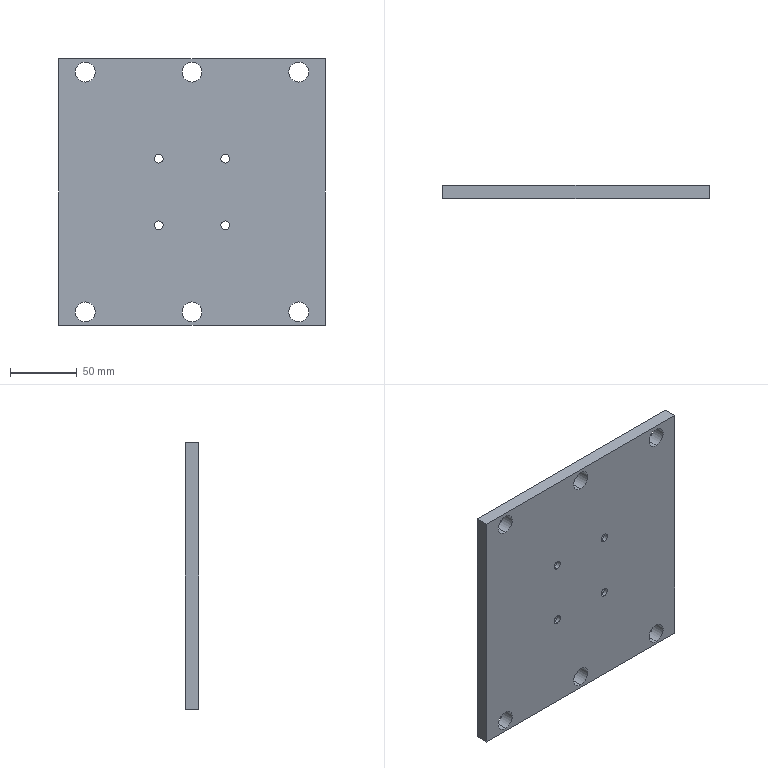Part | SolidWorks | features Extrusion 1, HoleWzd 1, ICE 1, LPattern 1 | 1 solid | 38 faces | box 200 x 10 x 200 mm | volume 386374 mm3 | cylinder 28 | plane 10 | commonest cylinder face diameters 15 x12 6.6 x8 11 x8
STEP:
#1=CARTESIAN_POINT('',(25.,-1.8,-30.5));
#2=VERTEX_POINT('',#1);
#3=CARTESIAN_POINT('',(25.,-1.8,-19.5));
#4=VERTEX_POINT('',#3);
#5=CARTESIAN_POINT('',(25.,-1.8,-25.));
#6=DIRECTION('',(0.,1.,0.));
#7=DIRECTION('',(0.,0.,1.));
#8=AXIS2_PLACEMENT_3D('',#5,#6,#7);
#9=CIRCLE('',#8,5.5);
#10=EDGE_CURVE('',#2,#4,#9,.T.);
#11=ORIENTED_EDGE('',*,*,#10,.F.);
#12=CARTESIAN_POINT('',(25.,5.,-30.5));
#13=VERTEX_POINT('',#12);
#14=CARTESIAN_POINT('',(25.,5.,-30.5));
#15=DIRECTION('',(0.,1.,0.));
#16=VECTOR('',#15,1000.);
#17=LINE('',#14,#16);
#18=EDGE_CURVE('',#2,#13,#17,.T.);
#19=ORIENTED_EDGE('',*,*,#18,.T.);
#20=CARTESIAN_POINT('',(25.,5.,-19.5));
#21=VERTEX_POINT('',#20);
#22=CARTESIAN_POINT('',(25.,5.,-25.));
#23=DIRECTION('',(0.,1.,0.));
#24=DIRECTION('',(0.,0.,1.));
#25=AXIS2_PLACEMENT_3D('',#22,#23,#24);
#26=CIRCLE('',#25,5.5);
#27=EDGE_CURVE('',#13,#21,#26,.T.);
#28=ORIENTED_EDGE('',*,*,#27,.T.);
#29=CARTESIAN_POINT('',(25.,5.,-19.5));
#30=DIRECTION('',(0.,1.,0.));
#31=VECTOR('',#30,1000.);
#32=LINE('',#29,#31);
#33=EDGE_CURVE('',#4,#21,#32,.T.);
#34=ORIENTED_EDGE('',*,*,#33,.F.);
#35=EDGE_LOOP('',(#11,#19,#28,#34));
#36=FACE_OUTER_BOUND('',#35,.T.);
#37=CARTESIAN_POINT('',(25.,5.,-25.));
#38=DIRECTION('',(0.,1.,0.));
#39=DIRECTION('',(0.,0.,1.));
#40=AXIS2_PLACEMENT_3D('',#37,#38,#39);
#41=CYLINDRICAL_SURFACE('',#40,5.5);
#42=ADVANCED_FACE('',(#36),#41,.F.);
#43=CARTESIAN_POINT('',(25.,-5.,-28.3));
#44=VERTEX_POINT('',#43);
#45=CARTESIAN_POINT('',(25.,-5.,-21.7));
#46=VERTEX_POINT('',#45);
#47=CARTESIAN_POINT('',(25.,-5.,-25.));
#48=DIRECTION('',(0.,1.,0.));
#49=DIRECTION('',(0.,0.,1.));
#50=AXIS2_PLACEMENT_3D('',#47,#48,#49);
#51=CIRCLE('',#50,3.3);
#52=EDGE_CURVE('',#44,#46,#51,.T.);
#53=ORIENTED_EDGE('',*,*,#52,.F.);
#54=CARTESIAN_POINT('',(25.,-1.8,-28.3));
#55=VERTEX_POINT('',#54);
#56=CARTESIAN_POINT('',(25.,5.,-28.3));
#57=DIRECTION('',(0.,1.,0.));
#58=VECTOR('',#57,1000.);
#59=LINE('',#56,#58);
#60=EDGE_CURVE('',#44,#55,#59,.T.);
#61=ORIENTED_EDGE('',*,*,#60,.T.);
#62=CARTESIAN_POINT('',(25.,-1.8,-21.7));
#63=VERTEX_POINT('',#62);
#64=CARTESIAN_POINT('',(25.,-1.8,-25.));
#65=DIRECTION('',(0.,1.,0.));
#66=DIRECTION('',(0.,0.,1.));
#67=AXIS2_PLACEMENT_3D('',#64,#65,#66);
#68=CIRCLE('',#67,3.3);
#69=EDGE_CURVE('',#55,#63,#68,.T.);
#70=ORIENTED_EDGE('',*,*,#69,.T.);
#71=CARTESIAN_POINT('',(25.,5.,-21.7));
#72=DIRECTION('',(0.,1.,0.));
#73=VECTOR('',#72,1000.);
#74=LINE('',#71,#73);
#75=EDGE_CURVE('',#46,#63,#74,.T.);
#76=ORIENTED_EDGE('',*,*,#75,.F.);
#77=EDGE_LOOP('',(#53,#61,#70,#76));
#78=FACE_OUTER_BOUND('',#77,.T.);
#79=CARTESIAN_POINT('',(25.,5.,-25.));
#80=DIRECTION('',(0.,1.,0.));
#81=DIRECTION('',(0.,0.,1.));
#82=AXIS2_PLACEMENT_3D('',#79,#80,#81);
#83=CYLINDRICAL_SURFACE('',#82,3.3);
#84=ADVANCED_FACE('',(#78),#83,.F.);
#85=CARTESIAN_POINT('',(25.,-1.8,19.5));
#86=VERTEX_POINT('',#85);
#87=CARTESIAN_POINT('',(25.,-1.8,30.5));
#88=VERTEX_POINT('',#87);
#89=CARTESIAN_POINT('',(25.,-1.8,25.));
#90=DIRECTION('',(0.,1.,0.));
#91=DIRECTION('',(0.,0.,1.));
#92=AXIS2_PLACEMENT_3D('',#89,#90,#91);
#93=CIRCLE('',#92,5.5);
#94=EDGE_CURVE('',#86,#88,#93,.T.);
#95=ORIENTED_EDGE('',*,*,#94,.F.);
#96=CARTESIAN_POINT('',(25.,5.,19.5));
#97=VERTEX_POINT('',#96);
#98=CARTESIAN_POINT('',(25.,5.,19.5));
#99=DIRECTION('',(0.,1.,0.));
#100=VECTOR('',#99,1000.);
#101=LINE('',#98,#100);
#102=EDGE_CURVE('',#86,#97,#101,.T.);
#103=ORIENTED_EDGE('',*,*,#102,.T.);
#104=CARTESIAN_POINT('',(25.,5.,30.5));
#105=VERTEX_POINT('',#104);
#106=CARTESIAN_POINT('',(25.,5.,25.));
#107=DIRECTION('',(0.,1.,0.));
#108=DIRECTION('',(0.,0.,1.));
#109=AXIS2_PLACEMENT_3D('',#106,#107,#108);
#110=CIRCLE('',#109,5.5);
#111=EDGE_CURVE('',#97,#105,#110,.T.);
#112=ORIENTED_EDGE('',*,*,#111,.T.);
#113=CARTESIAN_POINT('',(25.,5.,30.5));
#114=DIRECTION('',(0.,1.,0.));
#115=VECTOR('',#114,1000.);
#116=LINE('',#113,#115);
#117=EDGE_CURVE('',#88,#105,#116,.T.);
#118=ORIENTED_EDGE('',*,*,#117,.F.);
#119=EDGE_LOOP('',(#95,#103,#112,#118));
#120=FACE_OUTER_BOUND('',#119,.T.);
#121=CARTESIAN_POINT('',(25.,5.,25.));
#122=DIRECTION('',(0.,1.,0.));
#123=DIRECTION('',(0.,0.,1.));
#124=AXIS2_PLACEMENT_3D('',#121,#122,#123);
#125=CYLINDRICAL_SURFACE('',#124,5.5);
#126=ADVANCED_FACE('',(#120),#125,.F.);
#127=CARTESIAN_POINT('',(25.,-5.,21.7));
#128=VERTEX_POINT('',#127);
#129=CARTESIAN_POINT('',(25.,-5.,28.3));
#130=VERTEX_POINT('',#129);
#131=CARTESIAN_POINT('',(25.,-5.,25.));
#132=DIRECTION('',(0.,1.,0.));
#133=DIRECTION('',(0.,0.,1.));
#134=AXIS2_PLACEMENT_3D('',#131,#132,#133);
#135=CIRCLE('',#134,3.3);
#136=EDGE_CURVE('',#128,#130,#135,.T.);
#137=ORIENTED_EDGE('',*,*,#136,.F.);
#138=CARTESIAN_POINT('',(25.,-1.8,21.7));
#139=VERTEX_POINT('',#138);
#140=CARTESIAN_POINT('',(25.,5.,21.7));
#141=DIRECTION('',(0.,1.,0.));
#142=VECTOR('',#141,1000.);
#143=LINE('',#140,#142);
#144=EDGE_CURVE('',#128,#139,#143,.T.);
#145=ORIENTED_EDGE('',*,*,#144,.T.);
#146=CARTESIAN_POINT('',(25.,-1.8,28.3));
#147=VERTEX_POINT('',#146);
#148=CARTESIAN_POINT('',(25.,-1.8,25.));
#149=DIRECTION('',(0.,1.,0.));
#150=DIRECTION('',(0.,0.,1.));
#151=AXIS2_PLACEMENT_3D('',#148,#149,#150);
#152=CIRCLE('',#151,3.3);
#153=EDGE_CURVE('',#139,#147,#152,.T.);
#154=ORIENTED_EDGE('',*,*,#153,.T.);
#155=CARTESIAN_POINT('',(25.,5.,28.3));
#156=DIRECTION('',(0.,1.,0.));
#157=VECTOR('',#156,1000.);
#158=LINE('',#155,#157);
#159=EDGE_CURVE('',#130,#147,#158,.T.);
#160=ORIENTED_EDGE('',*,*,#159,.F.);
#161=EDGE_LOOP('',(#137,#145,#154,#160));
#162=FACE_OUTER_BOUND('',#161,.T.);
#163=CARTESIAN_POINT('',(25.,5.,25.));
#164=DIRECTION('',(0.,1.,0.));
#165=DIRECTION('',(0.,0.,1.));
#166=AXIS2_PLACEMENT_3D('',#163,#164,#165);
#167=CYLINDRICAL_SURFACE('',#166,3.3);
#168=ADVANCED_FACE('',(#162),#167,.F.);
#169=CARTESIAN_POINT('',(-25.,-1.8,-30.5));
#170=VERTEX_POINT('',#169);
#171=CARTESIAN_POINT('',(-25.,-1.8,-19.5));
#172=VERTEX_POINT('',#171);
#173=CARTESIAN_POINT('',(-25.,-1.8,-25.));
#174=DIRECTION('',(0.,1.,0.));
#175=DIRECTION('',(0.,0.,1.));
#176=AXIS2_PLACEMENT_3D('',#173,#174,#175);
#177=CIRCLE('',#176,5.5);
#178=EDGE_CURVE('',#170,#172,#177,.T.);
#179=ORIENTED_EDGE('',*,*,#178,.F.);
#180=CARTESIAN_POINT('',(-25.,5.,-30.5));
#181=VERTEX_POINT('',#180);
#182=CARTESIAN_POINT('',(-25.,5.,-30.5));
#183=DIRECTION('',(0.,1.,0.));
#184=VECTOR('',#183,1000.);
#185=LINE('',#182,#184);
#186=EDGE_CURVE('',#170,#181,#185,.T.);
#187=ORIENTED_EDGE('',*,*,#186,.T.);
#188=CARTESIAN_POINT('',(-25.,5.,-19.5));
#189=VERTEX_POINT('',#188);
#190=CARTESIAN_POINT('',(-25.,5.,-25.));
#191=DIRECTION('',(0.,1.,0.));
#192=DIRECTION('',(0.,0.,1.));
#193=AXIS2_PLACEMENT_3D('',#190,#191,#192);
#194=CIRCLE('',#193,5.5);
#195=EDGE_CURVE('',#181,#189,#194,.T.);
#196=ORIENTED_EDGE('',*,*,#195,.T.);
#197=CARTESIAN_POINT('',(-25.,5.,-19.5));
#198=DIRECTION('',(0.,1.,0.));
#199=VECTOR('',#198,1000.);
#200=LINE('',#197,#199);
#201=EDGE_CURVE('',#172,#189,#200,.T.);
#202=ORIENTED_EDGE('',*,*,#201,.F.);
#203=EDGE_LOOP('',(#179,#187,#196,#202));
#204=FACE_OUTER_BOUND('',#203,.T.);
#205=CARTESIAN_POINT('',(-25.,5.,-25.));
#206=DIRECTION('',(0.,1.,0.));
#207=DIRECTION('',(0.,0.,1.));
#208=AXIS2_PLACEMENT_3D('',#205,#206,#207);
#209=CYLINDRICAL_SURFACE('',#208,5.5);
#210=ADVANCED_FACE('',(#204),#209,.F.);
#211=CARTESIAN_POINT('',(-25.,-5.,-28.3));
#212=VERTEX_POINT('',#211);
#213=CARTESIAN_POINT('',(-25.,-5.,-21.7));
#214=VERTEX_POINT('',#213);
#215=CARTESIAN_POINT('',(-25.,-5.,-25.));
#216=DIRECTION('',(0.,1.,0.));
#217=DIRECTION('',(0.,0.,1.));
#218=AXIS2_PLACEMENT_3D('',#215,#216,#217);
#219=CIRCLE('',#218,3.3);
#220=EDGE_CURVE('',#212,#214,#219,.T.);
#221=ORIENTED_EDGE('',*,*,#220,.F.);
#222=CARTESIAN_POINT('',(-25.,-1.8,-28.3));
#223=VERTEX_POINT('',#222);
#224=CARTESIAN_POINT('',(-25.,5.,-28.3));
#225=DIRECTION('',(0.,1.,0.));
#226=VECTOR('',#225,1000.);
#227=LINE('',#224,#226);
#228=EDGE_CURVE('',#212,#223,#227,.T.);
#229=ORIENTED_EDGE('',*,*,#228,.T.);
#230=CARTESIAN_POINT('',(-25.,-1.8,-21.7));
#231=VERTEX_POINT('',#230);
#232=CARTESIAN_POINT('',(-25.,-1.8,-25.));
#233=DIRECTION('',(0.,1.,0.));
#234=DIRECTION('',(0.,0.,1.));
#235=AXIS2_PLACEMENT_3D('',#232,#233,#234);
#236=CIRCLE('',#235,3.3);
#237=EDGE_CURVE('',#223,#231,#236,.T.);
#238=ORIENTED_EDGE('',*,*,#237,.T.);
#239=CARTESIAN_POINT('',(-25.,5.,-21.7));
#240=DIRECTION('',(0.,1.,0.));
#241=VECTOR('',#240,1000.);
#242=LINE('',#239,#241);
#243=EDGE_CURVE('',#214,#231,#242,.T.);
#244=ORIENTED_EDGE('',*,*,#243,.F.);
#245=EDGE_LOOP('',(#221,#229,#238,#244));
#246=FACE_OUTER_BOUND('',#245,.T.);
#247=CARTESIAN_POINT('',(-25.,5.,-25.));
#248=DIRECTION('',(0.,1.,0.));
#249=DIRECTION('',(0.,0.,1.));
#250=AXIS2_PLACEMENT_3D('',#247,#248,#249);
#251=CYLINDRICAL_SURFACE('',#250,3.3);
#252=ADVANCED_FACE('',(#246),#251,.F.);
#253=CARTESIAN_POINT('',(-25.,-1.8,19.5));
#254=VERTEX_POINT('',#253);
#255=CARTESIAN_POINT('',(-25.,-1.8,30.5));
#256=VERTEX_POINT('',#255);
#257=CARTESIAN_POINT('',(-25.,-1.8,25.));
#258=DIRECTION('',(0.,1.,0.));
#259=DIRECTION('',(0.,0.,1.));
#260=AXIS2_PLACEMENT_3D('',#257,#258,#259);
#261=CIRCLE('',#260,5.5);
#262=EDGE_CURVE('',#254,#256,#261,.T.);
#263=ORIENTED_EDGE('',*,*,#262,.F.);
#264=CARTESIAN_POINT('',(-25.,5.,19.5));
#265=VERTEX_POINT('',#264);
#266=CARTESIAN_POINT('',(-25.,5.,19.5));
#267=DIRECTION('',(0.,1.,0.));
#268=VECTOR('',#267,1000.);
#269=LINE('',#266,#268);
#270=EDGE_CURVE('',#254,#265,#269,.T.);
#271=ORIENTED_EDGE('',*,*,#270,.T.);
#272=CARTESIAN_POINT('',(-25.,5.,30.5));
#273=VERTEX_POINT('',#272);
#274=CARTESIAN_POINT('',(-25.,5.,25.));
#275=DIRECTION('',(0.,1.,0.));
#276=DIRECTION('',(0.,0.,1.));
#277=AXIS2_PLACEMENT_3D('',#274,#275,#276);
#278=CIRCLE('',#277,5.5);
#279=EDGE_CURVE('',#265,#273,#278,.T.);
#280=ORIENTED_EDGE('',*,*,#279,.T.);
#281=CARTESIAN_POINT('',(-25.,5.,30.5));
#282=DIRECTION('',(0.,1.,0.));
#283=VECTOR('',#282,1000.);
#284=LINE('',#281,#283);
#285=EDGE_CURVE('',#256,#273,#284,.T.);
#286=ORIENTED_EDGE('',*,*,#285,.F.);
#287=EDGE_LOOP('',(#263,#271,#280,#286));
#288=FACE_OUTER_BOUND('',#287,.T.);
#289=CARTESIAN_POINT('',(-25.,5.,25.));
#290=DIRECTION('',(0.,1.,0.));
#291=DIRECTION('',(0.,0.,1.));
#292=AXIS2_PLACEMENT_3D('',#289,#290,#291);
#293=CYLINDRICAL_SURFACE('',#292,5.5);
#294=ADVANCED_FACE('',(#288),#293,.F.);
#295=CARTESIAN_POINT('',(-25.,-5.,21.7));
#296=VERTEX_POINT('',#295);
#297=CARTESIAN_POINT('',(-25.,-5.,28.3));
#298=VERTEX_POINT('',#297);
#299=CARTESIAN_POINT('',(-25.,-5.,25.));
#300=DIRECTION('',(0.,1.,0.));
#301=DIRECTION('',(0.,0.,1.));
#302=AXIS2_PLACEMENT_3D('',#299,#300,#301);
#303=CIRCLE('',#302,3.3);
#304=EDGE_CURVE('',#296,#298,#303,.T.);
#305=ORIENTED_EDGE('',*,*,#304,.F.);
#306=CARTESIAN_POINT('',(-25.,-1.8,21.7));
#307=VERTEX_POINT('',#306);
#308=CARTESIAN_POINT('',(-25.,5.,21.7));
#309=DIRECTION('',(0.,1.,0.));
#310=VECTOR('',#309,1000.);
#311=LINE('',#308,#310);
#312=EDGE_CURVE('',#296,#307,#311,.T.);
#313=ORIENTED_EDGE('',*,*,#312,.T.);
#314=CARTESIAN_POINT('',(-25.,-1.8,28.3));
#315=VERTEX_POINT('',#314);
#316=CARTESIAN_POINT('',(-25.,-1.8,25.));
#317=DIRECTION('',(0.,1.,0.));
#318=DIRECTION('',(0.,0.,1.));
#319=AXIS2_PLACEMENT_3D('',#316,#317,#318);
#320=CIRCLE('',#319,3.3);
#321=EDGE_CURVE('',#307,#315,#320,.T.);
#322=ORIENTED_EDGE('',*,*,#321,.T.);
#323=CARTESIAN_POINT('',(-25.,5.,28.3));
#324=DIRECTION('',(0.,1.,0.));
#325=VECTOR('',#324,1000.);
#326=LINE('',#323,#325);
#327=EDGE_CURVE('',#298,#315,#326,.T.);
#328=ORIENTED_EDGE('',*,*,#327,.F.);
#329=EDGE_LOOP('',(#305,#313,#322,#328));
#330=FACE_OUTER_BOUND('',#329,.T.);
#331=CARTESIAN_POINT('',(-25.,5.,25.));
#332=DIRECTION('',(0.,1.,0.));
#333=DIRECTION('',(0.,0.,1.));
#334=AXIS2_PLACEMENT_3D('',#331,#332,#333);
#335=CYLINDRICAL_SURFACE('',#334,3.3);
#336=ADVANCED_FACE('',(#330),#335,.F.);
#337=CARTESIAN_POINT('',(80.,-5.,82.5));
#338=VERTEX_POINT('',#337);
#339=CARTESIAN_POINT('',(80.,-5.,97.5));
#340=VERTEX_POINT('',#339);
#341=CARTESIAN_POINT('',(80.,-5.,90.));
#342=DIRECTION('',(0.,1.,0.));
#343=DIRECTION('',(0.,0.,1.));
#344=AXIS2_PLACEMENT_3D('',#341,#342,#343);
#345=CIRCLE('',#344,7.5);
#346=EDGE_CURVE('',#338,#340,#345,.T.);
#347=ORIENTED_EDGE('',*,*,#346,.F.);
#348=CARTESIAN_POINT('',(80.,5.,82.5));
#349=VERTEX_POINT('',#348);
#350=CARTESIAN_POINT('',(80.,-5.,82.5));
#351=DIRECTION('',(0.,1.,0.));
#352=VECTOR('',#351,1000.);
#353=LINE('',#350,#352);
#354=EDGE_CURVE('',#338,#349,#353,.T.);
#355=ORIENTED_EDGE('',*,*,#354,.T.);
#356=CARTESIAN_POINT('',(80.,5.,97.5));
#357=VERTEX_POINT('',#356);
#358=CARTESIAN_POINT('',(80.,5.,90.));
#359=DIRECTION('',(0.,1.,0.));
#360=DIRECTION('',(0.,0.,1.));
#361=AXIS2_PLACEMENT_3D('',#358,#359,#360);
#362=CIRCLE('',#361,7.5);
#363=EDGE_CURVE('',#349,#357,#362,.T.);
#364=ORIENTED_EDGE('',*,*,#363,.T.);
#365=CARTESIAN_POINT('',(80.,-5.,97.5));
#366=DIRECTION('',(0.,1.,0.));
#367=VECTOR('',#366,1000.);
#368=LINE('',#365,#367);
#369=EDGE_CURVE('',#340,#357,#368,.T.);
#370=ORIENTED_EDGE('',*,*,#369,.F.);
#371=EDGE_LOOP('',(#347,#355,#364,#370));
#372=FACE_OUTER_BOUND('',#371,.T.);
#373=CARTESIAN_POINT('',(80.,-5.,90.));
#374=DIRECTION('',(0.,1.,0.));
#375=DIRECTION('',(0.,0.,1.));
#376=AXIS2_PLACEMENT_3D('',#373,#374,#375);
#377=CYLINDRICAL_SURFACE('',#376,7.5);
#378=ADVANCED_FACE('',(#372),#377,.F.);
#379=CARTESIAN_POINT('',(80.,-5.,-97.5));
#380=VERTEX_POINT('',#379);
#381=CARTESIAN_POINT('',(80.,-5.,-82.5));
#382=VERTEX_POINT('',#381);
#383=CARTESIAN_POINT('',(80.,-5.,-90.));
#384=DIRECTION('',(0.,1.,0.));
#385=DIRECTION('',(0.,0.,1.));
#386=AXIS2_PLACEMENT_3D('',#383,#384,#385);
#387=CIRCLE('',#386,7.5);
#388=EDGE_CURVE('',#380,#382,#387,.T.);
#389=ORIENTED_EDGE('',*,*,#388,.F.);
#390=CARTESIAN_POINT('',(80.,5.,-97.5));
#391=VERTEX_POINT('',#390);
#392=CARTESIAN_POINT('',(80.,-5.,-97.5));
#393=DIRECTION('',(0.,1.,0.));
#394=VECTOR('',#393,1000.);
#395=LINE('',#392,#394);
#396=EDGE_CURVE('',#380,#391,#395,.T.);
#397=ORIENTED_EDGE('',*,*,#396,.T.);
#398=CARTESIAN_POINT('',(80.,5.,-82.5));
#399=VERTEX_POINT('',#398);
#400=CARTESIAN_POINT('',(80.,5.,-90.));
#401=DIRECTION('',(0.,1.,0.));
#402=DIRECTION('',(0.,0.,1.));
#403=AXIS2_PLACEMENT_3D('',#400,#401,#402);
#404=CIRCLE('',#403,7.5);
#405=EDGE_CURVE('',#391,#399,#404,.T.);
#406=ORIENTED_EDGE('',*,*,#405,.T.);
#407=CARTESIAN_POINT('',(80.,-5.,-82.5));
#408=DIRECTION('',(0.,1.,0.));
#409=VECTOR('',#408,1000.);
#410=LINE('',#407,#409);
#411=EDGE_CURVE('',#382,#399,#410,.T.);
#412=ORIENTED_EDGE('',*,*,#411,.F.);
#413=EDGE_LOOP('',(#389,#397,#406,#412));
#414=FACE_OUTER_BOUND('',#413,.T.);
#415=CARTESIAN_POINT('',(80.,-5.,-90.));
#416=DIRECTION('',(0.,1.,0.));
#417=DIRECTION('',(0.,0.,1.));
#418=AXIS2_PLACEMENT_3D('',#415,#416,#417);
#419=CYLINDRICAL_SURFACE('',#418,7.5);
#420=ADVANCED_FACE('',(#414),#419,.F.);
#421=CARTESIAN_POINT('',(0.,-5.,-97.5));
#422=VERTEX_POINT('',#421);
#423=CARTESIAN_POINT('',(0.,-5.,-82.5));
#424=VERTEX_POINT('',#423);
#425=CARTESIAN_POINT('',(0.,-5.,-90.));
#426=DIRECTION('',(0.,1.,0.));
#427=DIRECTION('',(0.,0.,1.));
#428=AXIS2_PLACEMENT_3D('',#425,#426,#427);
#429=CIRCLE('',#428,7.5);
#430=EDGE_CURVE('',#422,#424,#429,.T.);
#431=ORIENTED_EDGE('',*,*,#430,.F.);
#432=CARTESIAN_POINT('',(0.,5.,-97.5));
#433=VERTEX_POINT('',#432);
#434=CARTESIAN_POINT('',(0.,-5.,-97.5));
#435=DIRECTION('',(0.,1.,0.));
#436=VECTOR('',#435,1000.);
#437=LINE('',#434,#436);
#438=EDGE_CURVE('',#422,#433,#437,.T.);
#439=ORIENTED_EDGE('',*,*,#438,.T.);
#440=CARTESIAN_POINT('',(0.,5.,-82.5));
#441=VERTEX_POINT('',#440);
#442=CARTESIAN_POINT('',(0.,5.,-90.));
#443=DIRECTION('',(0.,1.,0.));
#444=DIRECTION('',(0.,0.,1.));
#445=AXIS2_PLACEMENT_3D('',#442,#443,#444);
#446=CIRCLE('',#445,7.5);
#447=EDGE_CURVE('',#433,#441,#446,.T.);
#448=ORIENTED_EDGE('',*,*,#447,.T.);
#449=CARTESIAN_POINT('',(0.,-5.,-82.5));
#450=DIRECTION('',(0.,1.,0.));
#451=VECTOR('',#450,1000.);
#452=LINE('',#449,#451);
#453=EDGE_CURVE('',#424,#441,#452,.T.);
#454=ORIENTED_EDGE('',*,*,#453,.F.);
#455=EDGE_LOOP('',(#431,#439,#448,#454));
#456=FACE_OUTER_BOUND('',#455,.T.);
#457=CARTESIAN_POINT('',(0.,-5.,-90.));
#458=DIRECTION('',(0.,1.,0.));
#459=DIRECTION('',(0.,0.,1.));
#460=AXIS2_PLACEMENT_3D('',#457,#458,#459);
#461=CYLINDRICAL_SURFACE('',#460,7.5);
#462=ADVANCED_FACE('',(#456),#461,.F.);
#463=CARTESIAN_POINT('',(0.,-5.,82.5));
#464=VERTEX_POINT('',#463);
#465=CARTESIAN_POINT('',(0.,-5.,97.5));
#466=VERTEX_POINT('',#465);
#467=CARTESIAN_POINT('',(0.,-5.,90.));
#468=DIRECTION('',(0.,1.,0.));
#469=DIRECTION('',(0.,0.,1.));
#470=AXIS2_PLACEMENT_3D('',#467,#468,#469);
#471=CIRCLE('',#470,7.5);
#472=EDGE_CURVE('',#464,#466,#471,.T.);
#473=ORIENTED_EDGE('',*,*,#472,.F.);
#474=CARTESIAN_POINT('',(0.,5.,82.5));
#475=VERTEX_POINT('',#474);
#476=CARTESIAN_POINT('',(0.,-5.,82.5));
#477=DIRECTION('',(0.,1.,0.));
#478=VECTOR('',#477,1000.);
#479=LINE('',#476,#478);
#480=EDGE_CURVE('',#464,#475,#479,.T.);
#481=ORIENTED_EDGE('',*,*,#480,.T.);
#482=CARTESIAN_POINT('',(0.,5.,97.5));
#483=VERTEX_POINT('',#482);
#484=CARTESIAN_POINT('',(0.,5.,90.));
#485=DIRECTION('',(0.,1.,0.));
#486=DIRECTION('',(0.,0.,1.));
#487=AXIS2_PLACEMENT_3D('',#484,#485,#486);
#488=CIRCLE('',#487,7.5);
#489=EDGE_CURVE('',#475,#483,#488,.T.);
#490=ORIENTED_EDGE('',*,*,#489,.T.);
#491=CARTESIAN_POINT('',(0.,-5.,97.5));
#492=DIRECTION('',(0.,1.,0.));
#493=VECTOR('',#492,1000.);
#494=LINE('',#491,#493);
#495=EDGE_CURVE('',#466,#483,#494,.T.);
#496=ORIENTED_EDGE('',*,*,#495,.F.);
#497=EDGE_LOOP('',(#473,#481,#490,#496));
#498=FACE_OUTER_BOUND('',#497,.T.);
#499=CARTESIAN_POINT('',(0.,-5.,90.));
#500=DIRECTION('',(0.,1.,0.));
#501=DIRECTION('',(0.,0.,1.));
#502=AXIS2_PLACEMENT_3D('',#499,#500,#501);
#503=CYLINDRICAL_SURFACE('',#502,7.5);
#504=ADVANCED_FACE('',(#498),#503,.F.);
#505=CARTESIAN_POINT('',(-80.,-5.,-97.5));
#506=VERTEX_POINT('',#505);
#507=CARTESIAN_POINT('',(-80.,-5.,-82.5));
#508=VERTEX_POINT('',#507);
#509=CARTESIAN_POINT('',(-80.,-5.,-90.));
#510=DIRECTION('',(0.,1.,0.));
#511=DIRECTION('',(0.,0.,1.));
#512=AXIS2_PLACEMENT_3D('',#509,#510,#511);
#513=CIRCLE('',#512,7.5);
#514=EDGE_CURVE('',#506,#508,#513,.T.);
#515=ORIENTED_EDGE('',*,*,#514,.F.);
#516=CARTESIAN_POINT('',(-80.,5.,-97.5));
#517=VERTEX_POINT('',#516);
#518=CARTESIAN_POINT('',(-80.,-5.,-97.5));
#519=DIRECTION('',(0.,1.,0.));
#520=VECTOR('',#519,1000.);
#521=LINE('',#518,#520);
#522=EDGE_CURVE('',#506,#517,#521,.T.);
#523=ORIENTED_EDGE('',*,*,#522,.T.);
#524=CARTESIAN_POINT('',(-80.,5.,-82.5));
#525=VERTEX_POINT('',#524);
#526=CARTESIAN_POINT('',(-80.,5.,-90.));
#527=DIRECTION('',(0.,1.,0.));
#528=DIRECTION('',(0.,0.,1.));
#529=AXIS2_PLACEMENT_3D('',#526,#527,#528);
#530=CIRCLE('',#529,7.5);
#531=EDGE_CURVE('',#517,#525,#530,.T.);
#532=ORIENTED_EDGE('',*,*,#531,.T.);
#533=CARTESIAN_POINT('',(-80.,-5.,-82.5));
#534=DIRECTION('',(0.,1.,0.));
#535=VECTOR('',#534,1000.);
#536=LINE('',#533,#535);
#537=EDGE_CURVE('',#508,#525,#536,.T.);
#538=ORIENTED_EDGE('',*,*,#537,.F.);
#539=EDGE_LOOP('',(#515,#523,#532,#538));
#540=FACE_OUTER_BOUND('',#539,.T.);
#541=CARTESIAN_POINT('',(-80.,-5.,-90.));
#542=DIRECTION('',(0.,1.,0.));
#543=DIRECTION('',(0.,0.,1.));
#544=AXIS2_PLACEMENT_3D('',#541,#542,#543);
#545=CYLINDRICAL_SURFACE('',#544,7.5);
#546=ADVANCED_FACE('',(#540),#545,.F.);
#547=CARTESIAN_POINT('',(-80.,-5.,82.5));
#548=VERTEX_POINT('',#547);
#549=CARTESIAN_POINT('',(-80.,-5.,97.5));
#550=VERTEX_POINT('',#549);
#551=CARTESIAN_POINT('',(-80.,-5.,90.));
#552=DIRECTION('',(0.,1.,0.));
#553=DIRECTION('',(0.,0.,1.));
#554=AXIS2_PLACEMENT_3D('',#551,#552,#553);
#555=CIRCLE('',#554,7.5);
#556=EDGE_CURVE('',#548,#550,#555,.T.);
#557=ORIENTED_EDGE('',*,*,#556,.F.);
#558=CARTESIAN_POINT('',(-80.,5.,82.5));
#559=VERTEX_POINT('',#558);
#560=CARTESIAN_POINT('',(-80.,-5.,82.5));
#561=DIRECTION('',(0.,1.,0.));
#562=VECTOR('',#561,1000.);
#563=LINE('',#560,#562);
#564=EDGE_CURVE('',#548,#559,#563,.T.);
#565=ORIENTED_EDGE('',*,*,#564,.T.);
#566=CARTESIAN_POINT('',(-80.,5.,97.5));
#567=VERTEX_POINT('',#566);
#568=CARTESIAN_POINT('',(-80.,5.,90.));
#569=DIRECTION('',(0.,1.,0.));
#570=DIRECTION('',(0.,0.,1.));
#571=AXIS2_PLACEMENT_3D('',#568,#569,#570);
#572=CIRCLE('',#571,7.5);
#573=EDGE_CURVE('',#559,#567,#572,.T.);
#574=ORIENTED_EDGE('',*,*,#573,.T.);
#575=CARTESIAN_POINT('',(-80.,-5.,97.5));
#576=DIRECTION('',(0.,1.,0.));
#577=VECTOR('',#576,1000.);
#578=LINE('',#575,#577);
#579=EDGE_CURVE('',#550,#567,#578,.T.);
#580=ORIENTED_EDGE('',*,*,#579,.F.);
#581=EDGE_LOOP('',(#557,#565,#574,#580));
#582=FACE_OUTER_BOUND('',#581,.T.);
#583=CARTESIAN_POINT('',(-80.,-5.,90.));
#584=DIRECTION('',(0.,1.,0.));
#585=DIRECTION('',(0.,0.,1.));
#586=AXIS2_PLACEMENT_3D('',#583,#584,#585);
#587=CYLINDRICAL_SURFACE('',#586,7.5);
#588=ADVANCED_FACE('',(#582),#587,.F.);
#589=ORIENTED_EDGE('',*,*,#564,.F.);
#590=CARTESIAN_POINT('',(-80.,-5.,90.));
#591=DIRECTION('',(0.,1.,0.));
#592=DIRECTION('',(0.,0.,1.));
#593=AXIS2_PLACEMENT_3D('',#590,#591,#592);
#594=CIRCLE('',#593,7.5);
#595=EDGE_CURVE('',#550,#548,#594,.T.);
#596=ORIENTED_EDGE('',*,*,#595,.F.);
#597=ORIENTED_EDGE('',*,*,#579,.T.);
#598=CARTESIAN_POINT('',(-80.,5.,90.));
#599=DIRECTION('',(0.,1.,0.));
#600=DIRECTION('',(0.,0.,1.));
#601=AXIS2_PLACEMENT_3D('',#598,#599,#600);
#602=CIRCLE('',#601,7.5);
#603=EDGE_CURVE('',#567,#559,#602,.T.);
#604=ORIENTED_EDGE('',*,*,#603,.T.);
#605=EDGE_LOOP('',(#589,#596,#597,#604));
#606=FACE_OUTER_BOUND('',#605,.T.);
#607=CARTESIAN_POINT('',(-80.,-5.,90.));
#608=DIRECTION('',(0.,1.,0.));
#609=DIRECTION('',(0.,0.,1.));
#610=AXIS2_PLACEMENT_3D('',#607,#608,#609);
#611=CYLINDRICAL_SURFACE('',#610,7.5);
#612=ADVANCED_FACE('',(#606),#611,.F.);
#613=ORIENTED_EDGE('',*,*,#522,.F.);
#614=CARTESIAN_POINT('',(-80.,-5.,-90.));
#615=DIRECTION('',(0.,1.,0.));
#616=DIRECTION('',(0.,0.,1.));
#617=AXIS2_PLACEMENT_3D('',#614,#615,#616);
#618=CIRCLE('',#617,7.5);
#619=EDGE_CURVE('',#508,#506,#618,.T.);
#620=ORIENTED_EDGE('',*,*,#619,.F.);
#621=ORIENTED_EDGE('',*,*,#537,.T.);
#622=CARTESIAN_POINT('',(-80.,5.,-90.));
#623=DIRECTION('',(0.,1.,0.));
#624=DIRECTION('',(0.,0.,1.));
#625=AXIS2_PLACEMENT_3D('',#622,#623,#624);
#626=CIRCLE('',#625,7.5);
#627=EDGE_CURVE('',#525,#517,#626,.T.);
#628=ORIENTED_EDGE('',*,*,#627,.T.);
#629=EDGE_LOOP('',(#613,#620,#621,#628));
#630=FACE_OUTER_BOUND('',#629,.T.);
#631=CARTESIAN_POINT('',(-80.,-5.,-90.));
#632=DIRECTION('',(0.,1.,0.));
#633=DIRECTION('',(0.,0.,1.));
#634=AXIS2_PLACEMENT_3D('',#631,#632,#633);
#635=CYLINDRICAL_SURFACE('',#634,7.5);
#636=ADVANCED_FACE('',(#630),#635,.F.);
#637=ORIENTED_EDGE('',*,*,#480,.F.);
#638=CARTESIAN_POINT('',(0.,-5.,90.));
#639=DIRECTION('',(0.,1.,0.));
#640=DIRECTION('',(0.,0.,1.));
#641=AXIS2_PLACEMENT_3D('',#638,#639,#640);
#642=CIRCLE('',#641,7.5);
#643=EDGE_CURVE('',#466,#464,#642,.T.);
#644=ORIENTED_EDGE('',*,*,#643,.F.);
#645=ORIENTED_EDGE('',*,*,#495,.T.);
#646=CARTESIAN_POINT('',(0.,5.,90.));
#647=DIRECTION('',(0.,1.,0.));
#648=DIRECTION('',(0.,0.,1.));
#649=AXIS2_PLACEMENT_3D('',#646,#647,#648);
#650=CIRCLE('',#649,7.5);
#651=EDGE_CURVE('',#483,#475,#650,.T.);
#652=ORIENTED_EDGE('',*,*,#651,.T.);
#653=EDGE_LOOP('',(#637,#644,#645,#652));
#654=FACE_OUTER_BOUND('',#653,.T.);
#655=CARTESIAN_POINT('',(0.,-5.,90.));
#656=DIRECTION('',(0.,1.,0.));
#657=DIRECTION('',(0.,0.,1.));
#658=AXIS2_PLACEMENT_3D('',#655,#656,#657);
#659=CYLINDRICAL_SURFACE('',#658,7.5);
#660=ADVANCED_FACE('',(#654),#659,.F.);
#661=ORIENTED_EDGE('',*,*,#438,.F.);
#662=CARTESIAN_POINT('',(0.,-5.,-90.));
#663=DIRECTION('',(0.,1.,0.));
#664=DIRECTION('',(0.,0.,1.));
#665=AXIS2_PLACEMENT_3D('',#662,#663,#664);
#666=CIRCLE('',#665,7.5);
#667=EDGE_CURVE('',#424,#422,#666,.T.);
#668=ORIENTED_EDGE('',*,*,#667,.F.);
#669=ORIENTED_EDGE('',*,*,#453,.T.);
#670=CARTESIAN_POINT('',(0.,5.,-90.));
#671=DIRECTION('',(0.,1.,0.));
#672=DIRECTION('',(0.,0.,1.));
#673=AXIS2_PLACEMENT_3D('',#670,#671,#672);
#674=CIRCLE('',#673,7.5);
#675=EDGE_CURVE('',#441,#433,#674,.T.);
#676=ORIENTED_EDGE('',*,*,#675,.T.);
#677=EDGE_LOOP('',(#661,#668,#669,#676));
#678=FACE_OUTER_BOUND('',#677,.T.);
#679=CARTESIAN_POINT('',(0.,-5.,-90.));
#680=DIRECTION('',(0.,1.,0.));
#681=DIRECTION('',(0.,0.,1.));
#682=AXIS2_PLACEMENT_3D('',#679,#680,#681);
#683=CYLINDRICAL_SURFACE('',#682,7.5);
#684=ADVANCED_FACE('',(#678),#683,.F.);
#685=CARTESIAN_POINT('',(100.,-5.,100.));
#686=VERTEX_POINT('',#685);
#687=CARTESIAN_POINT('',(100.,-5.,-100.));
#688=VERTEX_POINT('',#687);
#689=CARTESIAN_POINT('',(100.,-5.,-100.));
#690=DIRECTION('',(0.,0.,-1.));
#691=VECTOR('',#690,1000.);
#692=LINE('',#689,#691);
#693=EDGE_CURVE('',#686,#688,#692,.T.);
#694=ORIENTED_EDGE('',*,*,#693,.T.);
#695=CARTESIAN_POINT('',(100.,5.,-100.));
#696=VERTEX_POINT('',#695);
#697=CARTESIAN_POINT('',(100.,5.,-100.));
#698=DIRECTION('',(0.,-1.,0.));
#699=VECTOR('',#698,1000.);
#700=LINE('',#697,#699);
#701=EDGE_CURVE('',#696,#688,#700,.T.);
#702=ORIENTED_EDGE('',*,*,#701,.F.);
#703=CARTESIAN_POINT('',(100.,5.,100.));
#704=VERTEX_POINT('',#703);
#705=CARTESIAN_POINT('',(100.,5.,-100.));
#706=DIRECTION('',(0.,0.,-1.));
#707=VECTOR('',#706,1000.);
#708=LINE('',#705,#707);
#709=EDGE_CURVE('',#704,#696,#708,.T.);
#710=ORIENTED_EDGE('',*,*,#709,.F.);
#711=CARTESIAN_POINT('',(100.,5.,100.));
#712=DIRECTION('',(0.,-1.,0.));
#713=VECTOR('',#712,1000.);
#714=LINE('',#711,#713);
#715=EDGE_CURVE('',#704,#686,#714,.T.);
#716=ORIENTED_EDGE('',*,*,#715,.T.);
#717=EDGE_LOOP('',(#694,#702,#710,#716));
#718=FACE_OUTER_BOUND('',#717,.T.);
#719=CARTESIAN_POINT('',(100.,5.,-100.));
#720=DIRECTION('',(-1.,0.,0.));
#721=DIRECTION('',(0.,0.,1.));
#722=AXIS2_PLACEMENT_3D('',#719,#720,#721);
#723=PLANE('',#722);
#724=ADVANCED_FACE('',(#718),#723,.F.);
#725=CARTESIAN_POINT('',(-100.,-5.,-100.));
#726=VERTEX_POINT('',#725);
#727=CARTESIAN_POINT('',(-100.,-5.,-100.));
#728=DIRECTION('',(-1.,0.,0.));
#729=VECTOR('',#728,1000.);
#730=LINE('',#727,#729);
#731=EDGE_CURVE('',#688,#726,#730,.T.);
#732=ORIENTED_EDGE('',*,*,#731,.T.);
#733=CARTESIAN_POINT('',(-100.,5.,-100.));
#734=VERTEX_POINT('',#733);
#735=CARTESIAN_POINT('',(-100.,5.,-100.));
#736=DIRECTION('',(0.,-1.,0.));
#737=VECTOR('',#736,1000.);
#738=LINE('',#735,#737);
#739=EDGE_CURVE('',#734,#726,#738,.T.);
#740=ORIENTED_EDGE('',*,*,#739,.F.);
#741=CARTESIAN_POINT('',(-100.,5.,-100.));
#742=DIRECTION('',(-1.,0.,0.));
#743=VECTOR('',#742,1000.);
#744=LINE('',#741,#743);
#745=EDGE_CURVE('',#696,#734,#744,.T.);
#746=ORIENTED_EDGE('',*,*,#745,.F.);
#747=ORIENTED_EDGE('',*,*,#701,.T.);
#748=EDGE_LOOP('',(#732,#740,#746,#747));
#749=FACE_OUTER_BOUND('',#748,.T.);
#750=CARTESIAN_POINT('',(-100.,5.,-100.));
#751=DIRECTION('',(0.,0.,1.));
#752=DIRECTION('',(1.,0.,0.));
#753=AXIS2_PLACEMENT_3D('',#750,#751,#752);
#754=PLANE('',#753);
#755=ADVANCED_FACE('',(#749),#754,.F.);
#756=CARTESIAN_POINT('',(-100.,-5.,100.));
#757=VERTEX_POINT('',#756);
#758=CARTESIAN_POINT('',(-100.,-5.,-100.));
#759=DIRECTION('',(0.,0.,1.));
#760=VECTOR('',#759,1000.);
#761=LINE('',#758,#760);
#762=EDGE_CURVE('',#726,#757,#761,.T.);
#763=ORIENTED_EDGE('',*,*,#762,.T.);
#764=CARTESIAN_POINT('',(-100.,5.,100.));
#765=VERTEX_POINT('',#764);
#766=CARTESIAN_POINT('',(-100.,5.,100.));
#767=DIRECTION('',(0.,-1.,0.));
#768=VECTOR('',#767,1000.);
#769=LINE('',#766,#768);
#770=EDGE_CURVE('',#765,#757,#769,.T.);
#771=ORIENTED_EDGE('',*,*,#770,.F.);
#772=CARTESIAN_POINT('',(-100.,5.,-100.));
#773=DIRECTION('',(0.,0.,1.));
#774=VECTOR('',#773,1000.);
#775=LINE('',#772,#774);
#776=EDGE_CURVE('',#734,#765,#775,.T.);
#777=ORIENTED_EDGE('',*,*,#776,.F.);
#778=ORIENTED_EDGE('',*,*,#739,.T.);
#779=EDGE_LOOP('',(#763,#771,#777,#778));
#780=FACE_OUTER_BOUND('',#779,.T.);
#781=CARTESIAN_POINT('',(-100.,5.,-100.));
#782=DIRECTION('',(1.,0.,0.));
#783=DIRECTION('',(0.,0.,-1.));
#784=AXIS2_PLACEMENT_3D('',#781,#782,#783);
#785=PLANE('',#784);
#786=ADVANCED_FACE('',(#780),#785,.F.);
#787=CARTESIAN_POINT('',(-100.,-5.,100.));
#788=DIRECTION('',(1.,0.,0.));
#789=VECTOR('',#788,1000.);
#790=LINE('',#787,#789);
#791=EDGE_CURVE('',#757,#686,#790,.T.);
#792=ORIENTED_EDGE('',*,*,#791,.T.);
#793=ORIENTED_EDGE('',*,*,#715,.F.);
#794=CARTESIAN_POINT('',(-100.,5.,100.));
#795=DIRECTION('',(1.,0.,0.));
#796=VECTOR('',#795,1000.);
#797=LINE('',#794,#796);
#798=EDGE_CURVE('',#765,#704,#797,.T.);
#799=ORIENTED_EDGE('',*,*,#798,.F.);
#800=ORIENTED_EDGE('',*,*,#770,.T.);
#801=EDGE_LOOP('',(#792,#793,#799,#800));
#802=FACE_OUTER_BOUND('',#801,.T.);
#803=CARTESIAN_POINT('',(-100.,5.,100.));
#804=DIRECTION('',(0.,0.,-1.));
#805=DIRECTION('',(-1.,0.,0.));
#806=AXIS2_PLACEMENT_3D('',#803,#804,#805);
#807=PLANE('',#806);
#808=ADVANCED_FACE('',(#802),#807,.F.);
#809=CARTESIAN_POINT('',(25.,5.,-25.));
#810=DIRECTION('',(0.,1.,0.));
#811=DIRECTION('',(0.,0.,1.));
#812=AXIS2_PLACEMENT_3D('',#809,#810,#811);
#813=CIRCLE('',#812,5.5);
#814=EDGE_CURVE('',#21,#13,#813,.T.);
#815=ORIENTED_EDGE('',*,*,#814,.F.);
#816=ORIENTED_EDGE('',*,*,#27,.F.);
#817=EDGE_LOOP('',(#815,#816));
#818=FACE_BOUND('',#817,.T.);
#819=CARTESIAN_POINT('',(25.,5.,25.));
#820=DIRECTION('',(0.,1.,0.));
#821=DIRECTION('',(0.,0.,1.));
#822=AXIS2_PLACEMENT_3D('',#819,#820,#821);
#823=CIRCLE('',#822,5.5);
#824=EDGE_CURVE('',#105,#97,#823,.T.);
#825=ORIENTED_EDGE('',*,*,#824,.F.);
#826=ORIENTED_EDGE('',*,*,#111,.F.);
#827=EDGE_LOOP('',(#825,#826));
#828=FACE_BOUND('',#827,.T.);
#829=CARTESIAN_POINT('',(-25.,5.,-25.));
#830=DIRECTION('',(0.,1.,0.));
#831=DIRECTION('',(0.,0.,1.));
#832=AXIS2_PLACEMENT_3D('',#829,#830,#831);
#833=CIRCLE('',#832,5.5);
#834=EDGE_CURVE('',#189,#181,#833,.T.);
#835=ORIENTED_EDGE('',*,*,#834,.F.);
#836=ORIENTED_EDGE('',*,*,#195,.F.);
#837=EDGE_LOOP('',(#835,#836));
#838=FACE_BOUND('',#837,.T.);
#839=CARTESIAN_POINT('',(-25.,5.,25.));
#840=DIRECTION('',(0.,1.,0.));
#841=DIRECTION('',(0.,0.,1.));
#842=AXIS2_PLACEMENT_3D('',#839,#840,#841);
#843=CIRCLE('',#842,5.5);
#844=EDGE_CURVE('',#273,#265,#843,.T.);
#845=ORIENTED_EDGE('',*,*,#844,.F.);
#846=ORIENTED_EDGE('',*,*,#279,.F.);
#847=EDGE_LOOP('',(#845,#846));
#848=FACE_BOUND('',#847,.T.);
#849=CARTESIAN_POINT('',(80.,5.,90.));
#850=DIRECTION('',(0.,1.,0.));
#851=DIRECTION('',(0.,0.,1.));
#852=AXIS2_PLACEMENT_3D('',#849,#850,#851);
#853=CIRCLE('',#852,7.5);
#854=EDGE_CURVE('',#357,#349,#853,.T.);
#855=ORIENTED_EDGE('',*,*,#854,.F.);
#856=ORIENTED_EDGE('',*,*,#363,.F.);
#857=EDGE_LOOP('',(#855,#856));
#858=FACE_BOUND('',#857,.T.);
#859=CARTESIAN_POINT('',(80.,5.,-90.));
#860=DIRECTION('',(0.,1.,0.));
#861=DIRECTION('',(0.,0.,1.));
#862=AXIS2_PLACEMENT_3D('',#859,#860,#861);
#863=CIRCLE('',#862,7.5);
#864=EDGE_CURVE('',#399,#391,#863,.T.);
#865=ORIENTED_EDGE('',*,*,#864,.F.);
#866=ORIENTED_EDGE('',*,*,#405,.F.);
#867=EDGE_LOOP('',(#865,#866));
#868=FACE_BOUND('',#867,.T.);
#869=ORIENTED_EDGE('',*,*,#709,.T.);
#870=ORIENTED_EDGE('',*,*,#745,.T.);
#871=ORIENTED_EDGE('',*,*,#776,.T.);
#872=ORIENTED_EDGE('',*,*,#798,.T.);
#873=EDGE_LOOP('',(#869,#870,#871,#872));
#874=FACE_OUTER_BOUND('',#873,.T.);
#875=ORIENTED_EDGE('',*,*,#675,.F.);
#876=ORIENTED_EDGE('',*,*,#447,.F.);
#877=EDGE_LOOP('',(#875,#876));
#878=FACE_BOUND('',#877,.T.);
#879=ORIENTED_EDGE('',*,*,#651,.F.);
#880=ORIENTED_EDGE('',*,*,#489,.F.);
#881=EDGE_LOOP('',(#879,#880));
#882=FACE_BOUND('',#881,.T.);
#883=ORIENTED_EDGE('',*,*,#627,.F.);
#884=ORIENTED_EDGE('',*,*,#531,.F.);
#885=EDGE_LOOP('',(#883,#884));
#886=FACE_BOUND('',#885,.T.);
#887=ORIENTED_EDGE('',*,*,#603,.F.);
#888=ORIENTED_EDGE('',*,*,#573,.F.);
#889=EDGE_LOOP('',(#887,#888));
#890=FACE_BOUND('',#889,.T.);
#891=CARTESIAN_POINT('',(0.,5.,0.));
#892=DIRECTION('',(0.,1.,0.));
#893=DIRECTION('',(0.,0.,1.));
#894=AXIS2_PLACEMENT_3D('',#891,#892,#893);
#895=PLANE('',#894);
#896=ADVANCED_FACE('',(#818,#828,#838,#848,#858,#868,#874,#878,#882,#886,#890),#895,.T.);
#897=CARTESIAN_POINT('',(25.,-5.,-25.));
#898=DIRECTION('',(0.,1.,0.));
#899=DIRECTION('',(0.,0.,1.));
#900=AXIS2_PLACEMENT_3D('',#897,#898,#899);
#901=CIRCLE('',#900,3.3);
#902=EDGE_CURVE('',#46,#44,#901,.T.);
#903=ORIENTED_EDGE('',*,*,#902,.T.);
#904=ORIENTED_EDGE('',*,*,#52,.T.);
#905=EDGE_LOOP('',(#903,#904));
#906=FACE_BOUND('',#905,.T.);
#907=CARTESIAN_POINT('',(25.,-5.,25.));
#908=DIRECTION('',(0.,1.,0.));
#909=DIRECTION('',(0.,0.,1.));
#910=AXIS2_PLACEMENT_3D('',#907,#908,#909);
#911=CIRCLE('',#910,3.3);
#912=EDGE_CURVE('',#130,#128,#911,.T.);
#913=ORIENTED_EDGE('',*,*,#912,.T.);
#914=ORIENTED_EDGE('',*,*,#136,.T.);
#915=EDGE_LOOP('',(#913,#914));
#916=FACE_BOUND('',#915,.T.);
#917=CARTESIAN_POINT('',(-25.,-5.,-25.));
#918=DIRECTION('',(0.,1.,0.));
#919=DIRECTION('',(0.,0.,1.));
#920=AXIS2_PLACEMENT_3D('',#917,#918,#919);
#921=CIRCLE('',#920,3.3);
#922=EDGE_CURVE('',#214,#212,#921,.T.);
#923=ORIENTED_EDGE('',*,*,#922,.T.);
#924=ORIENTED_EDGE('',*,*,#220,.T.);
#925=EDGE_LOOP('',(#923,#924));
#926=FACE_BOUND('',#925,.T.);
#927=CARTESIAN_POINT('',(-25.,-5.,25.));
#928=DIRECTION('',(0.,1.,0.));
#929=DIRECTION('',(0.,0.,1.));
#930=AXIS2_PLACEMENT_3D('',#927,#928,#929);
#931=CIRCLE('',#930,3.3);
#932=EDGE_CURVE('',#298,#296,#931,.T.);
#933=ORIENTED_EDGE('',*,*,#932,.T.);
#934=ORIENTED_EDGE('',*,*,#304,.T.);
#935=EDGE_LOOP('',(#933,#934));
#936=FACE_BOUND('',#935,.T.);
#937=CARTESIAN_POINT('',(80.,-5.,90.));
#938=DIRECTION('',(0.,1.,0.));
#939=DIRECTION('',(0.,0.,1.));
#940=AXIS2_PLACEMENT_3D('',#937,#938,#939);
#941=CIRCLE('',#940,7.5);
#942=EDGE_CURVE('',#340,#338,#941,.T.);
#943=ORIENTED_EDGE('',*,*,#942,.T.);
#944=ORIENTED_EDGE('',*,*,#346,.T.);
#945=EDGE_LOOP('',(#943,#944));
#946=FACE_BOUND('',#945,.T.);
#947=CARTESIAN_POINT('',(80.,-5.,-90.));
#948=DIRECTION('',(0.,1.,0.));
#949=DIRECTION('',(0.,0.,1.));
#950=AXIS2_PLACEMENT_3D('',#947,#948,#949);
#951=CIRCLE('',#950,7.5);
#952=EDGE_CURVE('',#382,#380,#951,.T.);
#953=ORIENTED_EDGE('',*,*,#952,.T.);
#954=ORIENTED_EDGE('',*,*,#388,.T.);
#955=EDGE_LOOP('',(#953,#954));
#956=FACE_BOUND('',#955,.T.);
#957=ORIENTED_EDGE('',*,*,#693,.F.);
#958=ORIENTED_EDGE('',*,*,#791,.F.);
#959=ORIENTED_EDGE('',*,*,#762,.F.);
#960=ORIENTED_EDGE('',*,*,#731,.F.);
#961=EDGE_LOOP('',(#957,#958,#959,#960));
#962=FACE_OUTER_BOUND('',#961,.T.);
#963=ORIENTED_EDGE('',*,*,#667,.T.);
#964=ORIENTED_EDGE('',*,*,#430,.T.);
#965=EDGE_LOOP('',(#963,#964));
#966=FACE_BOUND('',#965,.T.);
#967=ORIENTED_EDGE('',*,*,#643,.T.);
#968=ORIENTED_EDGE('',*,*,#472,.T.);
#969=EDGE_LOOP('',(#967,#968));
#970=FACE_BOUND('',#969,.T.);
#971=ORIENTED_EDGE('',*,*,#619,.T.);
#972=ORIENTED_EDGE('',*,*,#514,.T.);
#973=EDGE_LOOP('',(#971,#972));
#974=FACE_BOUND('',#973,.T.);
#975=ORIENTED_EDGE('',*,*,#595,.T.);
#976=ORIENTED_EDGE('',*,*,#556,.T.);
#977=EDGE_LOOP('',(#975,#976));
#978=FACE_BOUND('',#977,.T.);
#979=CARTESIAN_POINT('',(0.,-5.,0.));
#980=DIRECTION('',(0.,1.,0.));
#981=DIRECTION('',(0.,0.,1.));
#982=AXIS2_PLACEMENT_3D('',#979,#980,#981);
#983=PLANE('',#982);
#984=ADVANCED_FACE('',(#906,#916,#926,#936,#946,#956,#962,#966,#970,#974,#978),#983,.F.);
#985=ORIENTED_EDGE('',*,*,#396,.F.);
#986=ORIENTED_EDGE('',*,*,#952,.F.);
#987=ORIENTED_EDGE('',*,*,#411,.T.);
#988=ORIENTED_EDGE('',*,*,#864,.T.);
#989=EDGE_LOOP('',(#985,#986,#987,#988));
#990=FACE_OUTER_BOUND('',#989,.T.);
#991=CARTESIAN_POINT('',(80.,-5.,-90.));
#992=DIRECTION('',(0.,1.,0.));
#993=DIRECTION('',(0.,0.,1.));
#994=AXIS2_PLACEMENT_3D('',#991,#992,#993);
#995=CYLINDRICAL_SURFACE('',#994,7.5);
#996=ADVANCED_FACE('',(#990),#995,.F.);
#997=ORIENTED_EDGE('',*,*,#354,.F.);
#998=ORIENTED_EDGE('',*,*,#942,.F.);
#999=ORIENTED_EDGE('',*,*,#369,.T.);
#1000=ORIENTED_EDGE('',*,*,#854,.T.);
#1001=EDGE_LOOP('',(#997,#998,#999,#1000));
#1002=FACE_OUTER_BOUND('',#1001,.T.);
#1003=CARTESIAN_POINT('',(80.,-5.,90.));
#1004=DIRECTION('',(0.,1.,0.));
#1005=DIRECTION('',(0.,0.,1.));
#1006=AXIS2_PLACEMENT_3D('',#1003,#1004,#1005);
#1007=CYLINDRICAL_SURFACE('',#1006,7.5);
#1008=ADVANCED_FACE('',(#1002),#1007,.F.);
#1009=ORIENTED_EDGE('',*,*,#312,.F.);
#1010=ORIENTED_EDGE('',*,*,#932,.F.);
#1011=ORIENTED_EDGE('',*,*,#327,.T.);
#1012=CARTESIAN_POINT('',(-25.,-1.8,25.));
#1013=DIRECTION('',(0.,1.,0.));
#1014=DIRECTION('',(0.,0.,1.));
#1015=AXIS2_PLACEMENT_3D('',#1012,#1013,#1014);
#1016=CIRCLE('',#1015,3.3);
#1017=EDGE_CURVE('',#315,#307,#1016,.T.);
#1018=ORIENTED_EDGE('',*,*,#1017,.T.);
#1019=EDGE_LOOP('',(#1009,#1010,#1011,#1018));
#1020=FACE_OUTER_BOUND('',#1019,.T.);
#1021=CARTESIAN_POINT('',(-25.,5.,25.));
#1022=DIRECTION('',(0.,1.,0.));
#1023=DIRECTION('',(0.,0.,1.));
#1024=AXIS2_PLACEMENT_3D('',#1021,#1022,#1023);
#1025=CYLINDRICAL_SURFACE('',#1024,3.3);
#1026=ADVANCED_FACE('',(#1020),#1025,.F.);
#1027=ORIENTED_EDGE('',*,*,#1017,.F.);
#1028=ORIENTED_EDGE('',*,*,#321,.F.);
#1029=EDGE_LOOP('',(#1027,#1028));
#1030=FACE_BOUND('',#1029,.T.);
#1031=CARTESIAN_POINT('',(-25.,-1.8,25.));
#1032=DIRECTION('',(0.,1.,0.));
#1033=DIRECTION('',(0.,0.,1.));
#1034=AXIS2_PLACEMENT_3D('',#1031,#1032,#1033);
#1035=CIRCLE('',#1034,5.5);
#1036=EDGE_CURVE('',#256,#254,#1035,.T.);
#1037=ORIENTED_EDGE('',*,*,#1036,.T.);
#1038=ORIENTED_EDGE('',*,*,#262,.T.);
#1039=EDGE_LOOP('',(#1037,#1038));
#1040=FACE_OUTER_BOUND('',#1039,.T.);
#1041=CARTESIAN_POINT('',(-21.7,-1.8,25.));
#1042=DIRECTION('',(0.,-1.,0.));
#1043=DIRECTION('',(0.,0.,-1.));
#1044=AXIS2_PLACEMENT_3D('',#1041,#1042,#1043);
#1045=PLANE('',#1044);
#1046=ADVANCED_FACE('',(#1030,#1040),#1045,.F.);
#1047=ORIENTED_EDGE('',*,*,#270,.F.);
#1048=ORIENTED_EDGE('',*,*,#1036,.F.);
#1049=ORIENTED_EDGE('',*,*,#285,.T.);
#1050=ORIENTED_EDGE('',*,*,#844,.T.);
#1051=EDGE_LOOP('',(#1047,#1048,#1049,#1050));
#1052=FACE_OUTER_BOUND('',#1051,.T.);
#1053=CARTESIAN_POINT('',(-25.,5.,25.));
#1054=DIRECTION('',(0.,1.,0.));
#1055=DIRECTION('',(0.,0.,1.));
#1056=AXIS2_PLACEMENT_3D('',#1053,#1054,#1055);
#1057=CYLINDRICAL_SURFACE('',#1056,5.5);
#1058=ADVANCED_FACE('',(#1052),#1057,.F.);
#1059=ORIENTED_EDGE('',*,*,#228,.F.);
#1060=ORIENTED_EDGE('',*,*,#922,.F.);
#1061=ORIENTED_EDGE('',*,*,#243,.T.);
#1062=CARTESIAN_POINT('',(-25.,-1.8,-25.));
#1063=DIRECTION('',(0.,1.,0.));
#1064=DIRECTION('',(0.,0.,1.));
#1065=AXIS2_PLACEMENT_3D('',#1062,#1063,#1064);
#1066=CIRCLE('',#1065,3.3);
#1067=EDGE_CURVE('',#231,#223,#1066,.T.);
#1068=ORIENTED_EDGE('',*,*,#1067,.T.);
#1069=EDGE_LOOP('',(#1059,#1060,#1061,#1068));
#1070=FACE_OUTER_BOUND('',#1069,.T.);
#1071=CARTESIAN_POINT('',(-25.,5.,-25.));
#1072=DIRECTION('',(0.,1.,0.));
#1073=DIRECTION('',(0.,0.,1.));
#1074=AXIS2_PLACEMENT_3D('',#1071,#1072,#1073);
#1075=CYLINDRICAL_SURFACE('',#1074,3.3);
#1076=ADVANCED_FACE('',(#1070),#1075,.F.);
#1077=ORIENTED_EDGE('',*,*,#1067,.F.);
#1078=ORIENTED_EDGE('',*,*,#237,.F.);
#1079=EDGE_LOOP('',(#1077,#1078));
#1080=FACE_BOUND('',#1079,.T.);
#1081=CARTESIAN_POINT('',(-25.,-1.8,-25.));
#1082=DIRECTION('',(0.,1.,0.));
#1083=DIRECTION('',(0.,0.,1.));
#1084=AXIS2_PLACEMENT_3D('',#1081,#1082,#1083);
#1085=CIRCLE('',#1084,5.5);
#1086=EDGE_CURVE('',#172,#170,#1085,.T.);
#1087=ORIENTED_EDGE('',*,*,#1086,.T.);
#1088=ORIENTED_EDGE('',*,*,#178,.T.);
#1089=EDGE_LOOP('',(#1087,#1088));
#1090=FACE_OUTER_BOUND('',#1089,.T.);
#1091=CARTESIAN_POINT('',(-21.7,-1.8,-25.));
#1092=DIRECTION('',(0.,-1.,0.));
#1093=DIRECTION('',(0.,0.,-1.));
#1094=AXIS2_PLACEMENT_3D('',#1091,#1092,#1093);
#1095=PLANE('',#1094);
#1096=ADVANCED_FACE('',(#1080,#1090),#1095,.F.);
#1097=ORIENTED_EDGE('',*,*,#186,.F.);
#1098=ORIENTED_EDGE('',*,*,#1086,.F.);
#1099=ORIENTED_EDGE('',*,*,#201,.T.);
#1100=ORIENTED_EDGE('',*,*,#834,.T.);
#1101=EDGE_LOOP('',(#1097,#1098,#1099,#1100));
#1102=FACE_OUTER_BOUND('',#1101,.T.);
#1103=CARTESIAN_POINT('',(-25.,5.,-25.));
#1104=DIRECTION('',(0.,1.,0.));
#1105=DIRECTION('',(0.,0.,1.));
#1106=AXIS2_PLACEMENT_3D('',#1103,#1104,#1105);
#1107=CYLINDRICAL_SURFACE('',#1106,5.5);
#1108=ADVANCED_FACE('',(#1102),#1107,.F.);
#1109=ORIENTED_EDGE('',*,*,#144,.F.);
#1110=ORIENTED_EDGE('',*,*,#912,.F.);
#1111=ORIENTED_EDGE('',*,*,#159,.T.);
#1112=CARTESIAN_POINT('',(25.,-1.8,25.));
#1113=DIRECTION('',(0.,1.,0.));
#1114=DIRECTION('',(0.,0.,1.));
#1115=AXIS2_PLACEMENT_3D('',#1112,#1113,#1114);
#1116=CIRCLE('',#1115,3.3);
#1117=EDGE_CURVE('',#147,#139,#1116,.T.);
#1118=ORIENTED_EDGE('',*,*,#1117,.T.);
#1119=EDGE_LOOP('',(#1109,#1110,#1111,#1118));
#1120=FACE_OUTER_BOUND('',#1119,.T.);
#1121=CARTESIAN_POINT('',(25.,5.,25.));
#1122=DIRECTION('',(0.,1.,0.));
#1123=DIRECTION('',(0.,0.,1.));
#1124=AXIS2_PLACEMENT_3D('',#1121,#1122,#1123);
#1125=CYLINDRICAL_SURFACE('',#1124,3.3);
#1126=ADVANCED_FACE('',(#1120),#1125,.F.);
#1127=ORIENTED_EDGE('',*,*,#1117,.F.);
#1128=ORIENTED_EDGE('',*,*,#153,.F.);
#1129=EDGE_LOOP('',(#1127,#1128));
#1130=FACE_BOUND('',#1129,.T.);
#1131=CARTESIAN_POINT('',(25.,-1.8,25.));
#1132=DIRECTION('',(0.,1.,0.));
#1133=DIRECTION('',(0.,0.,1.));
#1134=AXIS2_PLACEMENT_3D('',#1131,#1132,#1133);
#1135=CIRCLE('',#1134,5.5);
#1136=EDGE_CURVE('',#88,#86,#1135,.T.);
#1137=ORIENTED_EDGE('',*,*,#1136,.T.);
#1138=ORIENTED_EDGE('',*,*,#94,.T.);
#1139=EDGE_LOOP('',(#1137,#1138));
#1140=FACE_OUTER_BOUND('',#1139,.T.);
#1141=CARTESIAN_POINT('',(28.3,-1.8,25.));
#1142=DIRECTION('',(0.,-1.,0.));
#1143=DIRECTION('',(0.,0.,-1.));
#1144=AXIS2_PLACEMENT_3D('',#1141,#1142,#1143);
#1145=PLANE('',#1144);
#1146=ADVANCED_FACE('',(#1130,#1140),#1145,.F.);
#1147=ORIENTED_EDGE('',*,*,#102,.F.);
#1148=ORIENTED_EDGE('',*,*,#1136,.F.);
#1149=ORIENTED_EDGE('',*,*,#117,.T.);
#1150=ORIENTED_EDGE('',*,*,#824,.T.);
#1151=EDGE_LOOP('',(#1147,#1148,#1149,#1150));
#1152=FACE_OUTER_BOUND('',#1151,.T.);
#1153=CARTESIAN_POINT('',(25.,5.,25.));
#1154=DIRECTION('',(0.,1.,0.));
#1155=DIRECTION('',(0.,0.,1.));
#1156=AXIS2_PLACEMENT_3D('',#1153,#1154,#1155);
#1157=CYLINDRICAL_SURFACE('',#1156,5.5);
#1158=ADVANCED_FACE('',(#1152),#1157,.F.);
#1159=ORIENTED_EDGE('',*,*,#60,.F.);
#1160=ORIENTED_EDGE('',*,*,#902,.F.);
#1161=ORIENTED_EDGE('',*,*,#75,.T.);
#1162=CARTESIAN_POINT('',(25.,-1.8,-25.));
#1163=DIRECTION('',(0.,1.,0.));
#1164=DIRECTION('',(0.,0.,1.));
#1165=AXIS2_PLACEMENT_3D('',#1162,#1163,#1164);
#1166=CIRCLE('',#1165,3.3);
#1167=EDGE_CURVE('',#63,#55,#1166,.T.);
#1168=ORIENTED_EDGE('',*,*,#1167,.T.);
#1169=EDGE_LOOP('',(#1159,#1160,#1161,#1168));
#1170=FACE_OUTER_BOUND('',#1169,.T.);
#1171=CARTESIAN_POINT('',(25.,5.,-25.));
#1172=DIRECTION('',(0.,1.,0.));
#1173=DIRECTION('',(0.,0.,1.));
#1174=AXIS2_PLACEMENT_3D('',#1171,#1172,#1173);
#1175=CYLINDRICAL_SURFACE('',#1174,3.3);
#1176=ADVANCED_FACE('',(#1170),#1175,.F.);
#1177=ORIENTED_EDGE('',*,*,#1167,.F.);
#1178=ORIENTED_EDGE('',*,*,#69,.F.);
#1179=EDGE_LOOP('',(#1177,#1178));
#1180=FACE_BOUND('',#1179,.T.);
#1181=CARTESIAN_POINT('',(25.,-1.8,-25.));
#1182=DIRECTION('',(0.,1.,0.));
#1183=DIRECTION('',(0.,0.,1.));
#1184=AXIS2_PLACEMENT_3D('',#1181,#1182,#1183);
#1185=CIRCLE('',#1184,5.5);
#1186=EDGE_CURVE('',#4,#2,#1185,.T.);
#1187=ORIENTED_EDGE('',*,*,#1186,.T.);
#1188=ORIENTED_EDGE('',*,*,#10,.T.);
#1189=EDGE_LOOP('',(#1187,#1188));
#1190=FACE_OUTER_BOUND('',#1189,.T.);
#1191=CARTESIAN_POINT('',(28.3,-1.8,-25.));
#1192=DIRECTION('',(0.,-1.,0.));
#1193=DIRECTION('',(0.,0.,-1.));
#1194=AXIS2_PLACEMENT_3D('',#1191,#1192,#1193);
#1195=PLANE('',#1194);
#1196=ADVANCED_FACE('',(#1180,#1190),#1195,.F.);
#1197=ORIENTED_EDGE('',*,*,#18,.F.);
#1198=ORIENTED_EDGE('',*,*,#1186,.F.);
#1199=ORIENTED_EDGE('',*,*,#33,.T.);
#1200=ORIENTED_EDGE('',*,*,#814,.T.);
#1201=EDGE_LOOP('',(#1197,#1198,#1199,#1200));
#1202=FACE_OUTER_BOUND('',#1201,.T.);
#1203=CARTESIAN_POINT('',(25.,5.,-25.));
#1204=DIRECTION('',(0.,1.,0.));
#1205=DIRECTION('',(0.,0.,1.));
#1206=AXIS2_PLACEMENT_3D('',#1203,#1204,#1205);
#1207=CYLINDRICAL_SURFACE('',#1206,5.5);
#1208=ADVANCED_FACE('',(#1202),#1207,.F.);
#1209=CLOSED_SHELL('',(#42,#84,#126,#168,#210,#252,#294,#336,#378,#420,#462,#504,#546,#588,#612,#636,#660,#684,#724,#755,#786,#808,#896,#984,#996,#1008,#1026,#1046,#1058,#1076,#1096,#1108,#1126,#1146,#1158,#1176,#1196,#1208));
#1210=MANIFOLD_SOLID_BREP('',#1209);
#1211=CARTESIAN_POINT('',(0.,0.,0.));
#1212=DIRECTION('',(0.,0.,1.));
#1213=DIRECTION('',(1.,0.,0.));
#1214=AXIS2_PLACEMENT_3D('',#1211,#1212,#1213);
#1215=(LENGTH_UNIT()NAMED_UNIT(*)SI_UNIT(.MILLI.,.METRE.));
#1216=UNCERTAINTY_MEASURE_WITH_UNIT(LENGTH_MEASURE(0.00001),#1215,'','');
#1217=(NAMED_UNIT(*)PLANE_ANGLE_UNIT()SI_UNIT($,.RADIAN.));
#1218=(NAMED_UNIT(*)SI_UNIT($,.STERADIAN.)SOLID_ANGLE_UNIT());
#1219=(GEOMETRIC_REPRESENTATION_CONTEXT(3)GLOBAL_UNCERTAINTY_ASSIGNED_CONTEXT((#1216))GLOBAL_UNIT_ASSIGNED_CONTEXT((#1215,#1217,#1218))REPRESENTATION_CONTEXT('',''));
#1220=ADVANCED_BREP_SHAPE_REPRESENTATION('',(#1210,#1214),#1219);